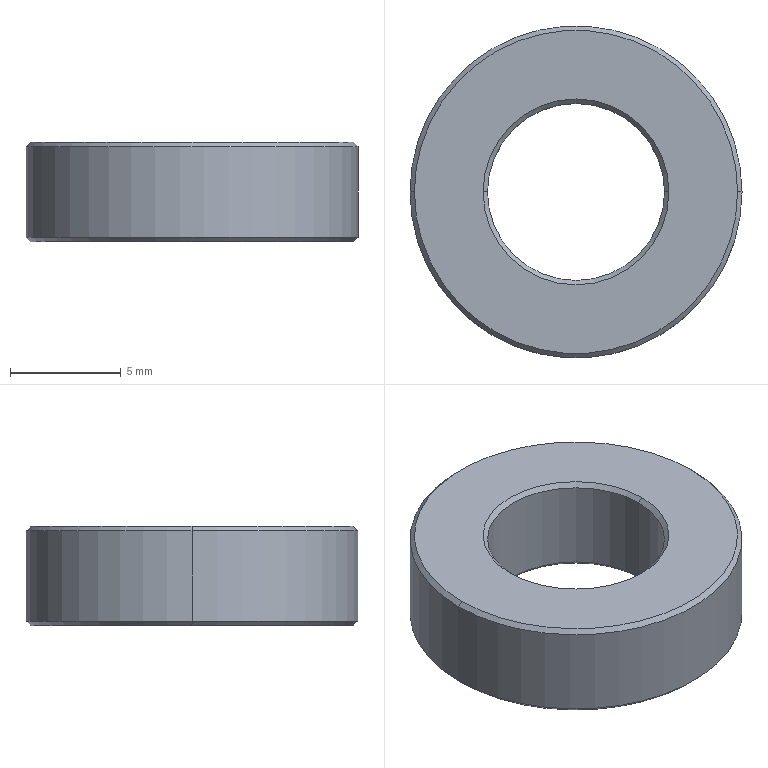Part | STEP file | 1 solid | 14 faces | box 15 x 15 x 4.5 mm | volume 566.131 mm3 | cone 8 | cylinder 4 | plane 2 | commonest cylinder face diameters 8 x2 15 x2
STEP:
#1=CARTESIAN_POINT('',(0.,0.,0.));
#2=DIRECTION('',(0.,0.,1.));
#3=DIRECTION('',(1.,0.,0.));
#4=AXIS2_PLACEMENT_3D('',#1,#2,#3);
#5=CARTESIAN_POINT('',(4.,0.,4.3));
#6=VERTEX_POINT('',#5);
#7=CARTESIAN_POINT('',(4.2,0.,4.5));
#8=VERTEX_POINT('',#7);
#9=CARTESIAN_POINT('',(4.,0.,4.3));
#10=DIRECTION('',(0.7071,0.,0.7071));
#11=VECTOR('',#10,1.);
#12=LINE('',#9,#11);
#13=CARTESIAN_POINT('',(0.,0.,4.3));
#14=DIRECTION('',(0.,0.,1.));
#15=DIRECTION('',(1.,0.,0.));
#16=AXIS2_PLACEMENT_3D('',#13,#14,#15);
#17=CONICAL_SURFACE('',#16,4.,0.7854);
#18=CARTESIAN_POINT('',(6.283,0.));
#19=DIRECTION('',(0.,1.));
#20=VECTOR('',#19,1.);
#21=LINE('',#18,#20);
#22=(GEOMETRIC_REPRESENTATION_CONTEXT(2)PARAMETRIC_REPRESENTATION_CONTEXT()REPRESENTATION_CONTEXT('',''));
#23=DEFINITIONAL_REPRESENTATION('',(#21),#22);
#24=PCURVE('',#17,#23);
#25=CARTESIAN_POINT('',(0.,0.,4.3));
#26=DIRECTION('',(0.,0.,1.));
#27=DIRECTION('',(1.,0.,0.));
#28=AXIS2_PLACEMENT_3D('',#25,#26,#27);
#29=CONICAL_SURFACE('',#28,4.,0.7854);
#30=CARTESIAN_POINT('',(0.,0.));
#31=DIRECTION('',(0.,1.));
#32=VECTOR('',#31,1.);
#33=LINE('',#30,#32);
#34=(GEOMETRIC_REPRESENTATION_CONTEXT(2)PARAMETRIC_REPRESENTATION_CONTEXT()REPRESENTATION_CONTEXT('',''));
#35=DEFINITIONAL_REPRESENTATION('',(#33),#34);
#36=PCURVE('',#29,#35);
#37=SURFACE_CURVE('',#12,(#24,#36),.PCURVE_S1.);
#38=EDGE_CURVE('',#6,#8,#37,.T.);
#39=ORIENTED_EDGE('',*,*,#38,.T.);
#40=CARTESIAN_POINT('',(-4.2,0.,4.5));
#41=VERTEX_POINT('',#40);
#42=CARTESIAN_POINT('',(0.,0.,4.5));
#43=DIRECTION('',(0.,0.,-1.));
#44=DIRECTION('',(1.,0.,0.));
#45=AXIS2_PLACEMENT_3D('',#42,#43,#44);
#46=CIRCLE('',#45,4.2);
#47=CARTESIAN_POINT('',(6.283,0.2));
#48=DIRECTION('',(-1.,0.));
#49=VECTOR('',#48,1.);
#50=LINE('',#47,#49);
#51=(GEOMETRIC_REPRESENTATION_CONTEXT(2)PARAMETRIC_REPRESENTATION_CONTEXT()REPRESENTATION_CONTEXT('',''));
#52=DEFINITIONAL_REPRESENTATION('',(#50),#51);
#53=PCURVE('',#17,#52);
#54=CARTESIAN_POINT('',(0.,0.,4.5));
#55=DIRECTION('',(0.,0.,1.));
#56=DIRECTION('',(1.,0.,0.));
#57=AXIS2_PLACEMENT_3D('',#54,#55,#56);
#58=PLANE('',#57);
#59=CARTESIAN_POINT('',(4.2,0.));
#60=CARTESIAN_POINT('',(4.2,-7.275));
#61=CARTESIAN_POINT('',(-2.1,-3.637));
#62=CARTESIAN_POINT('',(-8.4,0.));
#63=CARTESIAN_POINT('',(-2.1,3.637));
#64=CARTESIAN_POINT('',(4.2,7.275));
#65=CARTESIAN_POINT('',(4.2,0.));
#66=(BOUNDED_CURVE()B_SPLINE_CURVE(2,(#59,#60,#61,#62,#63,#64,#65),.UNSPECIFIED.,.T.,.F.)B_SPLINE_CURVE_WITH_KNOTS((1,2,2,2,2,1),(-2.094,0.,2.094,4.189,6.283,8.378),.UNSPECIFIED.)CURVE()GEOMETRIC_REPRESENTATION_ITEM()RATIONAL_B_SPLINE_CURVE((1.,0.5,1.,0.5,1.,0.5,1.))REPRESENTATION_ITEM(''));
#67=(GEOMETRIC_REPRESENTATION_CONTEXT(2)PARAMETRIC_REPRESENTATION_CONTEXT()REPRESENTATION_CONTEXT('',''));
#68=DEFINITIONAL_REPRESENTATION('',(#66),#67);
#69=PCURVE('',#58,#68);
#70=SURFACE_CURVE('',#46,(#53,#69),.PCURVE_S1.);
#71=EDGE_CURVE('',#8,#41,#70,.T.);
#72=ORIENTED_EDGE('',*,*,#71,.T.);
#73=CARTESIAN_POINT('',(-4.,0.,4.3));
#74=VERTEX_POINT('',#73);
#75=CARTESIAN_POINT('',(-4.,0.,4.3));
#76=DIRECTION('',(-0.7071,0.,0.7071));
#77=VECTOR('',#76,1.);
#78=LINE('',#75,#77);
#79=CARTESIAN_POINT('',(3.142,0.));
#80=DIRECTION('',(0.,1.));
#81=VECTOR('',#80,1.);
#82=LINE('',#79,#81);
#83=(GEOMETRIC_REPRESENTATION_CONTEXT(2)PARAMETRIC_REPRESENTATION_CONTEXT()REPRESENTATION_CONTEXT('',''));
#84=DEFINITIONAL_REPRESENTATION('',(#82),#83);
#85=PCURVE('',#17,#84);
#86=CARTESIAN_POINT('',(3.142,0.));
#87=DIRECTION('',(0.,1.));
#88=VECTOR('',#87,1.);
#89=LINE('',#86,#88);
#90=(GEOMETRIC_REPRESENTATION_CONTEXT(2)PARAMETRIC_REPRESENTATION_CONTEXT()REPRESENTATION_CONTEXT('',''));
#91=DEFINITIONAL_REPRESENTATION('',(#89),#90);
#92=PCURVE('',#29,#91);
#93=SURFACE_CURVE('',#78,(#85,#92),.PCURVE_S1.);
#94=EDGE_CURVE('',#74,#41,#93,.T.);
#95=ORIENTED_EDGE('',*,*,#94,.F.);
#96=CARTESIAN_POINT('',(0.,0.,4.3));
#97=DIRECTION('',(0.,0.,1.));
#98=DIRECTION('',(1.,0.,0.));
#99=AXIS2_PLACEMENT_3D('',#96,#97,#98);
#100=CIRCLE('',#99,4.);
#101=CARTESIAN_POINT('',(0.,0.));
#102=DIRECTION('',(1.,0.));
#103=VECTOR('',#102,1.);
#104=LINE('',#101,#103);
#105=(GEOMETRIC_REPRESENTATION_CONTEXT(2)PARAMETRIC_REPRESENTATION_CONTEXT()REPRESENTATION_CONTEXT('',''));
#106=DEFINITIONAL_REPRESENTATION('',(#104),#105);
#107=PCURVE('',#17,#106);
#108=CARTESIAN_POINT('',(0.,0.,4.5));
#109=DIRECTION('',(0.,0.,-1.));
#110=DIRECTION('',(-1.,0.,0.));
#111=AXIS2_PLACEMENT_3D('',#108,#109,#110);
#112=CYLINDRICAL_SURFACE('',#111,4.);
#113=CARTESIAN_POINT('',(9.425,0.2));
#114=DIRECTION('',(-1.,0.));
#115=VECTOR('',#114,1.);
#116=LINE('',#113,#115);
#117=(GEOMETRIC_REPRESENTATION_CONTEXT(2)PARAMETRIC_REPRESENTATION_CONTEXT()REPRESENTATION_CONTEXT('',''));
#118=DEFINITIONAL_REPRESENTATION('',(#116),#117);
#119=PCURVE('',#112,#118);
#120=SURFACE_CURVE('',#100,(#107,#119),.PCURVE_S1.);
#121=EDGE_CURVE('',#74,#6,#120,.T.);
#122=ORIENTED_EDGE('',*,*,#121,.T.);
#123=EDGE_LOOP('',(#39,#72,#95,#122));
#124=FACE_BOUND('',#123,.F.);
#125=ADVANCED_FACE('',(#124),#17,.F.);
#126=CARTESIAN_POINT('',(7.3,0.,4.5));
#127=VERTEX_POINT('',#126);
#128=CARTESIAN_POINT('',(-7.3,0.,4.5));
#129=VERTEX_POINT('',#128);
#130=CARTESIAN_POINT('',(0.,0.,4.5));
#131=DIRECTION('',(0.,0.,1.));
#132=DIRECTION('',(1.,0.,0.));
#133=AXIS2_PLACEMENT_3D('',#130,#131,#132);
#134=CIRCLE('',#133,7.3);
#135=CARTESIAN_POINT('',(0.,0.,4.5));
#136=DIRECTION('',(0.,0.,-1.));
#137=DIRECTION('',(-1.,0.,0.));
#138=AXIS2_PLACEMENT_3D('',#135,#136,#137);
#139=CONICAL_SURFACE('',#138,7.3,0.7854);
#140=CARTESIAN_POINT('',(3.142,0.));
#141=DIRECTION('',(-1.,0.));
#142=VECTOR('',#141,1.);
#143=LINE('',#140,#142);
#144=(GEOMETRIC_REPRESENTATION_CONTEXT(2)PARAMETRIC_REPRESENTATION_CONTEXT()REPRESENTATION_CONTEXT('',''));
#145=DEFINITIONAL_REPRESENTATION('',(#143),#144);
#146=PCURVE('',#139,#145);
#147=CARTESIAN_POINT('',(0.,0.));
#148=DIRECTION('',(1.,0.));
#149=AXIS2_PLACEMENT_2D('',#147,#148);
#150=CIRCLE('',#149,7.3);
#151=(GEOMETRIC_REPRESENTATION_CONTEXT(2)PARAMETRIC_REPRESENTATION_CONTEXT()REPRESENTATION_CONTEXT('',''));
#152=DEFINITIONAL_REPRESENTATION('',(#150),#151);
#153=PCURVE('',#58,#152);
#154=SURFACE_CURVE('',#134,(#146,#153),.PCURVE_S1.);
#155=EDGE_CURVE('',#127,#129,#154,.T.);
#156=ORIENTED_EDGE('',*,*,#155,.F.);
#157=CARTESIAN_POINT('',(7.5,0.,4.3));
#158=VERTEX_POINT('',#157);
#159=CARTESIAN_POINT('',(7.3,0.,4.5));
#160=DIRECTION('',(0.7071,0.,-0.7071));
#161=VECTOR('',#160,1.);
#162=LINE('',#159,#161);
#163=CARTESIAN_POINT('',(3.142,0.));
#164=DIRECTION('',(0.,1.));
#165=VECTOR('',#164,1.);
#166=LINE('',#163,#165);
#167=(GEOMETRIC_REPRESENTATION_CONTEXT(2)PARAMETRIC_REPRESENTATION_CONTEXT()REPRESENTATION_CONTEXT('',''));
#168=DEFINITIONAL_REPRESENTATION('',(#166),#167);
#169=PCURVE('',#139,#168);
#170=CARTESIAN_POINT('',(0.,0.,4.5));
#171=DIRECTION('',(0.,0.,-1.));
#172=DIRECTION('',(-1.,0.,0.));
#173=AXIS2_PLACEMENT_3D('',#170,#171,#172);
#174=CONICAL_SURFACE('',#173,7.3,0.7854);
#175=CARTESIAN_POINT('',(3.142,0.));
#176=DIRECTION('',(0.,1.));
#177=VECTOR('',#176,1.);
#178=LINE('',#175,#177);
#179=(GEOMETRIC_REPRESENTATION_CONTEXT(2)PARAMETRIC_REPRESENTATION_CONTEXT()REPRESENTATION_CONTEXT('',''));
#180=DEFINITIONAL_REPRESENTATION('',(#178),#179);
#181=PCURVE('',#174,#180);
#182=SURFACE_CURVE('',#162,(#169,#181),.PCURVE_S1.);
#183=EDGE_CURVE('',#127,#158,#182,.T.);
#184=ORIENTED_EDGE('',*,*,#183,.T.);
#185=CARTESIAN_POINT('',(-7.5,0.,4.3));
#186=VERTEX_POINT('',#185);
#187=CARTESIAN_POINT('',(0.,0.,4.3));
#188=DIRECTION('',(0.,0.,-1.));
#189=DIRECTION('',(1.,0.,0.));
#190=AXIS2_PLACEMENT_3D('',#187,#188,#189);
#191=CIRCLE('',#190,7.5);
#192=CARTESIAN_POINT('',(-3.142,0.2));
#193=DIRECTION('',(1.,0.));
#194=VECTOR('',#193,1.);
#195=LINE('',#192,#194);
#196=(GEOMETRIC_REPRESENTATION_CONTEXT(2)PARAMETRIC_REPRESENTATION_CONTEXT()REPRESENTATION_CONTEXT('',''));
#197=DEFINITIONAL_REPRESENTATION('',(#195),#196);
#198=PCURVE('',#139,#197);
#199=CARTESIAN_POINT('',(0.,0.,4.5));
#200=DIRECTION('',(0.,0.,-1.));
#201=DIRECTION('',(-1.,0.,0.));
#202=AXIS2_PLACEMENT_3D('',#199,#200,#201);
#203=CYLINDRICAL_SURFACE('',#202,7.5);
#204=CARTESIAN_POINT('',(-3.142,0.2));
#205=DIRECTION('',(1.,0.));
#206=VECTOR('',#205,1.);
#207=LINE('',#204,#206);
#208=(GEOMETRIC_REPRESENTATION_CONTEXT(2)PARAMETRIC_REPRESENTATION_CONTEXT()REPRESENTATION_CONTEXT('',''));
#209=DEFINITIONAL_REPRESENTATION('',(#207),#208);
#210=PCURVE('',#203,#209);
#211=SURFACE_CURVE('',#191,(#198,#210),.PCURVE_S1.);
#212=EDGE_CURVE('',#186,#158,#211,.T.);
#213=ORIENTED_EDGE('',*,*,#212,.F.);
#214=CARTESIAN_POINT('',(-7.3,0.,4.5));
#215=DIRECTION('',(-0.7071,0.,-0.7071));
#216=VECTOR('',#215,1.);
#217=LINE('',#214,#216);
#218=CARTESIAN_POINT('',(0.,0.));
#219=DIRECTION('',(0.,1.));
#220=VECTOR('',#219,1.);
#221=LINE('',#218,#220);
#222=(GEOMETRIC_REPRESENTATION_CONTEXT(2)PARAMETRIC_REPRESENTATION_CONTEXT()REPRESENTATION_CONTEXT('',''));
#223=DEFINITIONAL_REPRESENTATION('',(#221),#222);
#224=PCURVE('',#139,#223);
#225=CARTESIAN_POINT('',(6.283,0.));
#226=DIRECTION('',(0.,1.));
#227=VECTOR('',#226,1.);
#228=LINE('',#225,#227);
#229=(GEOMETRIC_REPRESENTATION_CONTEXT(2)PARAMETRIC_REPRESENTATION_CONTEXT()REPRESENTATION_CONTEXT('',''));
#230=DEFINITIONAL_REPRESENTATION('',(#228),#229);
#231=PCURVE('',#174,#230);
#232=SURFACE_CURVE('',#217,(#224,#231),.PCURVE_S1.);
#233=EDGE_CURVE('',#129,#186,#232,.T.);
#234=ORIENTED_EDGE('',*,*,#233,.F.);
#235=EDGE_LOOP('',(#156,#184,#213,#234));
#236=FACE_BOUND('',#235,.T.);
#237=ADVANCED_FACE('',(#236),#139,.T.);
#238=CARTESIAN_POINT('',(-7.3,0.,0.));
#239=VERTEX_POINT('',#238);
#240=CARTESIAN_POINT('',(7.3,0.,0.));
#241=VERTEX_POINT('',#240);
#242=CARTESIAN_POINT('',(0.,0.,0.));
#243=DIRECTION('',(0.,0.,-1.));
#244=DIRECTION('',(1.,0.,0.));
#245=AXIS2_PLACEMENT_3D('',#242,#243,#244);
#246=CIRCLE('',#245,7.3);
#247=CARTESIAN_POINT('',(0.,0.,0.2));
#248=DIRECTION('',(0.,0.,1.));
#249=DIRECTION('',(1.,0.,0.));
#250=AXIS2_PLACEMENT_3D('',#247,#248,#249);
#251=CONICAL_SURFACE('',#250,7.5,0.7854);
#252=CARTESIAN_POINT('',(6.283,-0.2));
#253=DIRECTION('',(-1.,0.));
#254=VECTOR('',#253,1.);
#255=LINE('',#252,#254);
#256=(GEOMETRIC_REPRESENTATION_CONTEXT(2)PARAMETRIC_REPRESENTATION_CONTEXT()REPRESENTATION_CONTEXT('',''));
#257=DEFINITIONAL_REPRESENTATION('',(#255),#256);
#258=PCURVE('',#251,#257);
#259=CARTESIAN_POINT('',(0.,0.,0.));
#260=DIRECTION('',(0.,0.,1.));
#261=DIRECTION('',(1.,0.,0.));
#262=AXIS2_PLACEMENT_3D('',#259,#260,#261);
#263=PLANE('',#262);
#264=CARTESIAN_POINT('',(7.3,0.));
#265=CARTESIAN_POINT('',(7.3,-12.644));
#266=CARTESIAN_POINT('',(-3.65,-6.322));
#267=CARTESIAN_POINT('',(-14.6,0.));
#268=CARTESIAN_POINT('',(-3.65,6.322));
#269=CARTESIAN_POINT('',(7.3,12.644));
#270=CARTESIAN_POINT('',(7.3,0.));
#271=(BOUNDED_CURVE()B_SPLINE_CURVE(2,(#264,#265,#266,#267,#268,#269,#270),.UNSPECIFIED.,.T.,.F.)B_SPLINE_CURVE_WITH_KNOTS((1,2,2,2,2,1),(-2.094,0.,2.094,4.189,6.283,8.378),.UNSPECIFIED.)CURVE()GEOMETRIC_REPRESENTATION_ITEM()RATIONAL_B_SPLINE_CURVE((1.,0.5,1.,0.5,1.,0.5,1.))REPRESENTATION_ITEM(''));
#272=(GEOMETRIC_REPRESENTATION_CONTEXT(2)PARAMETRIC_REPRESENTATION_CONTEXT()REPRESENTATION_CONTEXT('',''));
#273=DEFINITIONAL_REPRESENTATION('',(#271),#272);
#274=PCURVE('',#263,#273);
#275=SURFACE_CURVE('',#246,(#258,#274),.PCURVE_S1.);
#276=EDGE_CURVE('',#239,#241,#275,.T.);
#277=ORIENTED_EDGE('',*,*,#276,.F.);
#278=CARTESIAN_POINT('',(-7.5,0.,0.2));
#279=VERTEX_POINT('',#278);
#280=CARTESIAN_POINT('',(-7.5,0.,0.2));
#281=DIRECTION('',(-0.7071,0.,0.7071));
#282=VECTOR('',#281,1.);
#283=LINE('',#280,#282);
#284=CARTESIAN_POINT('',(3.142,0.));
#285=DIRECTION('',(0.,1.));
#286=VECTOR('',#285,1.);
#287=LINE('',#284,#286);
#288=(GEOMETRIC_REPRESENTATION_CONTEXT(2)PARAMETRIC_REPRESENTATION_CONTEXT()REPRESENTATION_CONTEXT('',''));
#289=DEFINITIONAL_REPRESENTATION('',(#287),#288);
#290=PCURVE('',#251,#289);
#291=CARTESIAN_POINT('',(0.,0.,0.2));
#292=DIRECTION('',(0.,0.,1.));
#293=DIRECTION('',(1.,0.,0.));
#294=AXIS2_PLACEMENT_3D('',#291,#292,#293);
#295=CONICAL_SURFACE('',#294,7.5,0.7854);
#296=CARTESIAN_POINT('',(3.142,0.));
#297=DIRECTION('',(0.,1.));
#298=VECTOR('',#297,1.);
#299=LINE('',#296,#298);
#300=(GEOMETRIC_REPRESENTATION_CONTEXT(2)PARAMETRIC_REPRESENTATION_CONTEXT()REPRESENTATION_CONTEXT('',''));
#301=DEFINITIONAL_REPRESENTATION('',(#299),#300);
#302=PCURVE('',#295,#301);
#303=SURFACE_CURVE('',#283,(#290,#302),.PCURVE_S1.);
#304=EDGE_CURVE('',#239,#279,#303,.T.);
#305=ORIENTED_EDGE('',*,*,#304,.T.);
#306=CARTESIAN_POINT('',(7.5,0.,0.2));
#307=VERTEX_POINT('',#306);
#308=CARTESIAN_POINT('',(0.,0.,0.2));
#309=DIRECTION('',(0.,0.,1.));
#310=DIRECTION('',(1.,0.,0.));
#311=AXIS2_PLACEMENT_3D('',#308,#309,#310);
#312=CIRCLE('',#311,7.5);
#313=CARTESIAN_POINT('',(0.,0.));
#314=DIRECTION('',(1.,0.));
#315=VECTOR('',#314,1.);
#316=LINE('',#313,#315);
#317=(GEOMETRIC_REPRESENTATION_CONTEXT(2)PARAMETRIC_REPRESENTATION_CONTEXT()REPRESENTATION_CONTEXT('',''));
#318=DEFINITIONAL_REPRESENTATION('',(#316),#317);
#319=PCURVE('',#251,#318);
#320=CARTESIAN_POINT('',(3.142,4.3));
#321=DIRECTION('',(-1.,0.));
#322=VECTOR('',#321,1.);
#323=LINE('',#320,#322);
#324=(GEOMETRIC_REPRESENTATION_CONTEXT(2)PARAMETRIC_REPRESENTATION_CONTEXT()REPRESENTATION_CONTEXT('',''));
#325=DEFINITIONAL_REPRESENTATION('',(#323),#324);
#326=PCURVE('',#203,#325);
#327=SURFACE_CURVE('',#312,(#319,#326),.PCURVE_S1.);
#328=EDGE_CURVE('',#307,#279,#327,.T.);
#329=ORIENTED_EDGE('',*,*,#328,.F.);
#330=CARTESIAN_POINT('',(7.5,0.,0.2));
#331=DIRECTION('',(0.7071,0.,0.7071));
#332=VECTOR('',#331,1.);
#333=LINE('',#330,#332);
#334=CARTESIAN_POINT('',(0.,0.));
#335=DIRECTION('',(0.,1.));
#336=VECTOR('',#335,1.);
#337=LINE('',#334,#336);
#338=(GEOMETRIC_REPRESENTATION_CONTEXT(2)PARAMETRIC_REPRESENTATION_CONTEXT()REPRESENTATION_CONTEXT('',''));
#339=DEFINITIONAL_REPRESENTATION('',(#337),#338);
#340=PCURVE('',#251,#339);
#341=CARTESIAN_POINT('',(6.283,0.));
#342=DIRECTION('',(0.,1.));
#343=VECTOR('',#342,1.);
#344=LINE('',#341,#343);
#345=(GEOMETRIC_REPRESENTATION_CONTEXT(2)PARAMETRIC_REPRESENTATION_CONTEXT()REPRESENTATION_CONTEXT('',''));
#346=DEFINITIONAL_REPRESENTATION('',(#344),#345);
#347=PCURVE('',#295,#346);
#348=SURFACE_CURVE('',#333,(#340,#347),.PCURVE_S1.);
#349=EDGE_CURVE('',#241,#307,#348,.T.);
#350=ORIENTED_EDGE('',*,*,#349,.F.);
#351=EDGE_LOOP('',(#277,#305,#329,#350));
#352=FACE_BOUND('',#351,.T.);
#353=ADVANCED_FACE('',(#352),#251,.T.);
#354=CARTESIAN_POINT('',(-4.,0.,0.2));
#355=VERTEX_POINT('',#354);
#356=CARTESIAN_POINT('',(-4.2,0.,0.));
#357=VERTEX_POINT('',#356);
#358=CARTESIAN_POINT('',(-4.2,0.,0.));
#359=DIRECTION('',(-0.7071,0.,-0.7071));
#360=VECTOR('',#359,1.);
#361=LINE('',#358,#360);
#362=CARTESIAN_POINT('',(0.,0.,0.));
#363=DIRECTION('',(0.,0.,-1.));
#364=DIRECTION('',(-1.,0.,0.));
#365=AXIS2_PLACEMENT_3D('',#362,#363,#364);
#366=CONICAL_SURFACE('',#365,4.2,0.7854);
#367=CARTESIAN_POINT('',(6.283,0.));
#368=DIRECTION('',(0.,1.));
#369=VECTOR('',#368,1.);
#370=LINE('',#367,#369);
#371=(GEOMETRIC_REPRESENTATION_CONTEXT(2)PARAMETRIC_REPRESENTATION_CONTEXT()REPRESENTATION_CONTEXT('',''));
#372=DEFINITIONAL_REPRESENTATION('',(#370),#371);
#373=PCURVE('',#366,#372);
#374=CARTESIAN_POINT('',(0.,0.,0.));
#375=DIRECTION('',(0.,0.,-1.));
#376=DIRECTION('',(-1.,0.,0.));
#377=AXIS2_PLACEMENT_3D('',#374,#375,#376);
#378=CONICAL_SURFACE('',#377,4.2,0.7854);
#379=CARTESIAN_POINT('',(0.,0.));
#380=DIRECTION('',(0.,1.));
#381=VECTOR('',#380,1.);
#382=LINE('',#379,#381);
#383=(GEOMETRIC_REPRESENTATION_CONTEXT(2)PARAMETRIC_REPRESENTATION_CONTEXT()REPRESENTATION_CONTEXT('',''));
#384=DEFINITIONAL_REPRESENTATION('',(#382),#383);
#385=PCURVE('',#378,#384);
#386=SURFACE_CURVE('',#361,(#373,#385),.PCURVE_S1.);
#387=EDGE_CURVE('',#355,#357,#386,.T.);
#388=ORIENTED_EDGE('',*,*,#387,.T.);
#389=CARTESIAN_POINT('',(4.2,0.,0.));
#390=VERTEX_POINT('',#389);
#391=CARTESIAN_POINT('',(0.,0.,0.));
#392=DIRECTION('',(0.,0.,1.));
#393=DIRECTION('',(1.,0.,0.));
#394=AXIS2_PLACEMENT_3D('',#391,#392,#393);
#395=CIRCLE('',#394,4.2);
#396=CARTESIAN_POINT('',(9.425,0.));
#397=DIRECTION('',(-1.,0.));
#398=VECTOR('',#397,1.);
#399=LINE('',#396,#398);
#400=(GEOMETRIC_REPRESENTATION_CONTEXT(2)PARAMETRIC_REPRESENTATION_CONTEXT()REPRESENTATION_CONTEXT('',''));
#401=DEFINITIONAL_REPRESENTATION('',(#399),#400);
#402=PCURVE('',#366,#401);
#403=CARTESIAN_POINT('',(0.,0.));
#404=DIRECTION('',(1.,0.));
#405=AXIS2_PLACEMENT_2D('',#403,#404);
#406=CIRCLE('',#405,4.2);
#407=(GEOMETRIC_REPRESENTATION_CONTEXT(2)PARAMETRIC_REPRESENTATION_CONTEXT()REPRESENTATION_CONTEXT('',''));
#408=DEFINITIONAL_REPRESENTATION('',(#406),#407);
#409=PCURVE('',#263,#408);
#410=SURFACE_CURVE('',#395,(#402,#409),.PCURVE_S1.);
#411=EDGE_CURVE('',#357,#390,#410,.T.);
#412=ORIENTED_EDGE('',*,*,#411,.T.);
#413=CARTESIAN_POINT('',(4.,0.,0.2));
#414=VERTEX_POINT('',#413);
#415=CARTESIAN_POINT('',(4.2,0.,0.));
#416=DIRECTION('',(0.7071,0.,-0.7071));
#417=VECTOR('',#416,1.);
#418=LINE('',#415,#417);
#419=CARTESIAN_POINT('',(3.142,0.));
#420=DIRECTION('',(0.,1.));
#421=VECTOR('',#420,1.);
#422=LINE('',#419,#421);
#423=(GEOMETRIC_REPRESENTATION_CONTEXT(2)PARAMETRIC_REPRESENTATION_CONTEXT()REPRESENTATION_CONTEXT('',''));
#424=DEFINITIONAL_REPRESENTATION('',(#422),#423);
#425=PCURVE('',#366,#424);
#426=CARTESIAN_POINT('',(3.142,0.));
#427=DIRECTION('',(0.,1.));
#428=VECTOR('',#427,1.);
#429=LINE('',#426,#428);
#430=(GEOMETRIC_REPRESENTATION_CONTEXT(2)PARAMETRIC_REPRESENTATION_CONTEXT()REPRESENTATION_CONTEXT('',''));
#431=DEFINITIONAL_REPRESENTATION('',(#429),#430);
#432=PCURVE('',#378,#431);
#433=SURFACE_CURVE('',#418,(#425,#432),.PCURVE_S1.);
#434=EDGE_CURVE('',#414,#390,#433,.T.);
#435=ORIENTED_EDGE('',*,*,#434,.F.);
#436=CARTESIAN_POINT('',(0.,0.,0.2));
#437=DIRECTION('',(0.,0.,-1.));
#438=DIRECTION('',(1.,0.,0.));
#439=AXIS2_PLACEMENT_3D('',#436,#437,#438);
#440=CIRCLE('',#439,4.);
#441=CARTESIAN_POINT('',(3.142,-0.2));
#442=DIRECTION('',(1.,0.));
#443=VECTOR('',#442,1.);
#444=LINE('',#441,#443);
#445=(GEOMETRIC_REPRESENTATION_CONTEXT(2)PARAMETRIC_REPRESENTATION_CONTEXT()REPRESENTATION_CONTEXT('',''));
#446=DEFINITIONAL_REPRESENTATION('',(#444),#445);
#447=PCURVE('',#366,#446);
#448=CARTESIAN_POINT('',(3.142,4.3));
#449=DIRECTION('',(1.,0.));
#450=VECTOR('',#449,1.);
#451=LINE('',#448,#450);
#452=(GEOMETRIC_REPRESENTATION_CONTEXT(2)PARAMETRIC_REPRESENTATION_CONTEXT()REPRESENTATION_CONTEXT('',''));
#453=DEFINITIONAL_REPRESENTATION('',(#451),#452);
#454=PCURVE('',#112,#453);
#455=SURFACE_CURVE('',#440,(#447,#454),.PCURVE_S1.);
#456=EDGE_CURVE('',#414,#355,#455,.T.);
#457=ORIENTED_EDGE('',*,*,#456,.T.);
#458=EDGE_LOOP('',(#388,#412,#435,#457));
#459=FACE_BOUND('',#458,.F.);
#460=ADVANCED_FACE('',(#459),#366,.F.);
#461=CARTESIAN_POINT('',(-4.,0.,4.5));
#462=DIRECTION('',(0.,0.,-1.));
#463=VECTOR('',#462,1.);
#464=LINE('',#461,#463);
#465=CARTESIAN_POINT('',(6.283,0.));
#466=DIRECTION('',(0.,1.));
#467=VECTOR('',#466,1.);
#468=LINE('',#465,#467);
#469=(GEOMETRIC_REPRESENTATION_CONTEXT(2)PARAMETRIC_REPRESENTATION_CONTEXT()REPRESENTATION_CONTEXT('',''));
#470=DEFINITIONAL_REPRESENTATION('',(#468),#469);
#471=PCURVE('',#112,#470);
#472=CARTESIAN_POINT('',(0.,0.,4.5));
#473=DIRECTION('',(0.,0.,-1.));
#474=DIRECTION('',(-1.,0.,0.));
#475=AXIS2_PLACEMENT_3D('',#472,#473,#474);
#476=CYLINDRICAL_SURFACE('',#475,4.);
#477=CARTESIAN_POINT('',(0.,0.));
#478=DIRECTION('',(0.,1.));
#479=VECTOR('',#478,1.);
#480=LINE('',#477,#479);
#481=(GEOMETRIC_REPRESENTATION_CONTEXT(2)PARAMETRIC_REPRESENTATION_CONTEXT()REPRESENTATION_CONTEXT('',''));
#482=DEFINITIONAL_REPRESENTATION('',(#480),#481);
#483=PCURVE('',#476,#482);
#484=SURFACE_CURVE('',#464,(#471,#483),.PCURVE_S1.);
#485=EDGE_CURVE('',#74,#355,#484,.T.);
#486=ORIENTED_EDGE('',*,*,#485,.T.);
#487=ORIENTED_EDGE('',*,*,#456,.F.);
#488=CARTESIAN_POINT('',(4.,0.,4.5));
#489=DIRECTION('',(0.,0.,-1.));
#490=VECTOR('',#489,1.);
#491=LINE('',#488,#490);
#492=CARTESIAN_POINT('',(3.142,0.));
#493=DIRECTION('',(0.,1.));
#494=VECTOR('',#493,1.);
#495=LINE('',#492,#494);
#496=(GEOMETRIC_REPRESENTATION_CONTEXT(2)PARAMETRIC_REPRESENTATION_CONTEXT()REPRESENTATION_CONTEXT('',''));
#497=DEFINITIONAL_REPRESENTATION('',(#495),#496);
#498=PCURVE('',#112,#497);
#499=CARTESIAN_POINT('',(3.142,0.));
#500=DIRECTION('',(0.,1.));
#501=VECTOR('',#500,1.);
#502=LINE('',#499,#501);
#503=(GEOMETRIC_REPRESENTATION_CONTEXT(2)PARAMETRIC_REPRESENTATION_CONTEXT()REPRESENTATION_CONTEXT('',''));
#504=DEFINITIONAL_REPRESENTATION('',(#502),#503);
#505=PCURVE('',#476,#504);
#506=SURFACE_CURVE('',#491,(#498,#505),.PCURVE_S1.);
#507=EDGE_CURVE('',#6,#414,#506,.T.);
#508=ORIENTED_EDGE('',*,*,#507,.F.);
#509=ORIENTED_EDGE('',*,*,#121,.F.);
#510=EDGE_LOOP('',(#486,#487,#508,#509));
#511=FACE_BOUND('',#510,.F.);
#512=ADVANCED_FACE('',(#511),#112,.F.);
#513=ORIENTED_EDGE('',*,*,#212,.T.);
#514=CARTESIAN_POINT('',(7.5,0.,4.5));
#515=DIRECTION('',(0.,0.,-1.));
#516=VECTOR('',#515,1.);
#517=LINE('',#514,#516);
#518=CARTESIAN_POINT('',(3.142,0.));
#519=DIRECTION('',(0.,1.));
#520=VECTOR('',#519,1.);
#521=LINE('',#518,#520);
#522=(GEOMETRIC_REPRESENTATION_CONTEXT(2)PARAMETRIC_REPRESENTATION_CONTEXT()REPRESENTATION_CONTEXT('',''));
#523=DEFINITIONAL_REPRESENTATION('',(#521),#522);
#524=PCURVE('',#203,#523);
#525=CARTESIAN_POINT('',(0.,0.,4.5));
#526=DIRECTION('',(0.,0.,-1.));
#527=DIRECTION('',(-1.,0.,0.));
#528=AXIS2_PLACEMENT_3D('',#525,#526,#527);
#529=CYLINDRICAL_SURFACE('',#528,7.5);
#530=CARTESIAN_POINT('',(3.142,0.));
#531=DIRECTION('',(0.,1.));
#532=VECTOR('',#531,1.);
#533=LINE('',#530,#532);
#534=(GEOMETRIC_REPRESENTATION_CONTEXT(2)PARAMETRIC_REPRESENTATION_CONTEXT()REPRESENTATION_CONTEXT('',''));
#535=DEFINITIONAL_REPRESENTATION('',(#533),#534);
#536=PCURVE('',#529,#535);
#537=SURFACE_CURVE('',#517,(#524,#536),.PCURVE_S1.);
#538=EDGE_CURVE('',#158,#307,#537,.T.);
#539=ORIENTED_EDGE('',*,*,#538,.T.);
#540=ORIENTED_EDGE('',*,*,#328,.T.);
#541=CARTESIAN_POINT('',(-7.5,0.,4.5));
#542=DIRECTION('',(0.,0.,-1.));
#543=VECTOR('',#542,1.);
#544=LINE('',#541,#543);
#545=CARTESIAN_POINT('',(0.,0.));
#546=DIRECTION('',(0.,1.));
#547=VECTOR('',#546,1.);
#548=LINE('',#545,#547);
#549=(GEOMETRIC_REPRESENTATION_CONTEXT(2)PARAMETRIC_REPRESENTATION_CONTEXT()REPRESENTATION_CONTEXT('',''));
#550=DEFINITIONAL_REPRESENTATION('',(#548),#549);
#551=PCURVE('',#203,#550);
#552=CARTESIAN_POINT('',(6.283,0.));
#553=DIRECTION('',(0.,1.));
#554=VECTOR('',#553,1.);
#555=LINE('',#552,#554);
#556=(GEOMETRIC_REPRESENTATION_CONTEXT(2)PARAMETRIC_REPRESENTATION_CONTEXT()REPRESENTATION_CONTEXT('',''));
#557=DEFINITIONAL_REPRESENTATION('',(#555),#556);
#558=PCURVE('',#529,#557);
#559=SURFACE_CURVE('',#544,(#551,#558),.PCURVE_S1.);
#560=EDGE_CURVE('',#186,#279,#559,.T.);
#561=ORIENTED_EDGE('',*,*,#560,.F.);
#562=EDGE_LOOP('',(#513,#539,#540,#561));
#563=FACE_BOUND('',#562,.T.);
#564=ADVANCED_FACE('',(#563),#203,.T.);
#565=CARTESIAN_POINT('',(0.,0.,4.5));
#566=DIRECTION('',(0.,0.,1.));
#567=DIRECTION('',(1.,0.,0.));
#568=AXIS2_PLACEMENT_3D('',#565,#566,#567);
#569=CIRCLE('',#568,7.3);
#570=CARTESIAN_POINT('',(0.,0.));
#571=DIRECTION('',(1.,0.));
#572=AXIS2_PLACEMENT_2D('',#570,#571);
#573=CIRCLE('',#572,7.3);
#574=(GEOMETRIC_REPRESENTATION_CONTEXT(2)PARAMETRIC_REPRESENTATION_CONTEXT()REPRESENTATION_CONTEXT('',''));
#575=DEFINITIONAL_REPRESENTATION('',(#573),#574);
#576=PCURVE('',#58,#575);
#577=CARTESIAN_POINT('',(9.425,0.));
#578=DIRECTION('',(-1.,0.));
#579=VECTOR('',#578,1.);
#580=LINE('',#577,#579);
#581=(GEOMETRIC_REPRESENTATION_CONTEXT(2)PARAMETRIC_REPRESENTATION_CONTEXT()REPRESENTATION_CONTEXT('',''));
#582=DEFINITIONAL_REPRESENTATION('',(#580),#581);
#583=PCURVE('',#174,#582);
#584=SURFACE_CURVE('',#569,(#576,#583),.PCURVE_S1.);
#585=EDGE_CURVE('',#129,#127,#584,.T.);
#586=ORIENTED_EDGE('',*,*,#585,.T.);
#587=ORIENTED_EDGE('',*,*,#155,.T.);
#588=EDGE_LOOP('',(#586,#587));
#589=FACE_BOUND('',#588,.T.);
#590=ORIENTED_EDGE('',*,*,#71,.T.);
#591=CARTESIAN_POINT('',(0.,0.,4.5));
#592=DIRECTION('',(0.,0.,-1.));
#593=DIRECTION('',(1.,0.,0.));
#594=AXIS2_PLACEMENT_3D('',#591,#592,#593);
#595=CIRCLE('',#594,4.2);
#596=CARTESIAN_POINT('',(4.2,0.));
#597=CARTESIAN_POINT('',(4.2,-7.275));
#598=CARTESIAN_POINT('',(-2.1,-3.637));
#599=CARTESIAN_POINT('',(-8.4,0.));
#600=CARTESIAN_POINT('',(-2.1,3.637));
#601=CARTESIAN_POINT('',(4.2,7.275));
#602=CARTESIAN_POINT('',(4.2,0.));
#603=(BOUNDED_CURVE()B_SPLINE_CURVE(2,(#596,#597,#598,#599,#600,#601,#602),.UNSPECIFIED.,.T.,.F.)B_SPLINE_CURVE_WITH_KNOTS((1,2,2,2,2,1),(-2.094,0.,2.094,4.189,6.283,8.378),.UNSPECIFIED.)CURVE()GEOMETRIC_REPRESENTATION_ITEM()RATIONAL_B_SPLINE_CURVE((1.,0.5,1.,0.5,1.,0.5,1.))REPRESENTATION_ITEM(''));
#604=(GEOMETRIC_REPRESENTATION_CONTEXT(2)PARAMETRIC_REPRESENTATION_CONTEXT()REPRESENTATION_CONTEXT('',''));
#605=DEFINITIONAL_REPRESENTATION('',(#603),#604);
#606=PCURVE('',#58,#605);
#607=CARTESIAN_POINT('',(6.283,0.2));
#608=DIRECTION('',(-1.,0.));
#609=VECTOR('',#608,1.);
#610=LINE('',#607,#609);
#611=(GEOMETRIC_REPRESENTATION_CONTEXT(2)PARAMETRIC_REPRESENTATION_CONTEXT()REPRESENTATION_CONTEXT('',''));
#612=DEFINITIONAL_REPRESENTATION('',(#610),#611);
#613=PCURVE('',#29,#612);
#614=SURFACE_CURVE('',#595,(#606,#613),.PCURVE_S1.);
#615=EDGE_CURVE('',#41,#8,#614,.T.);
#616=ORIENTED_EDGE('',*,*,#615,.T.);
#617=EDGE_LOOP('',(#590,#616));
#618=FACE_BOUND('',#617,.T.);
#619=ADVANCED_FACE('',(#589,#618),#58,.T.);
#620=ORIENTED_EDGE('',*,*,#411,.T.);
#621=CARTESIAN_POINT('',(0.,0.,0.));
#622=DIRECTION('',(0.,0.,1.));
#623=DIRECTION('',(1.,0.,0.));
#624=AXIS2_PLACEMENT_3D('',#621,#622,#623);
#625=CIRCLE('',#624,4.2);
#626=CARTESIAN_POINT('',(0.,0.));
#627=DIRECTION('',(1.,0.));
#628=AXIS2_PLACEMENT_2D('',#626,#627);
#629=CIRCLE('',#628,4.2);
#630=(GEOMETRIC_REPRESENTATION_CONTEXT(2)PARAMETRIC_REPRESENTATION_CONTEXT()REPRESENTATION_CONTEXT('',''));
#631=DEFINITIONAL_REPRESENTATION('',(#629),#630);
#632=PCURVE('',#263,#631);
#633=CARTESIAN_POINT('',(3.142,0.));
#634=DIRECTION('',(-1.,0.));
#635=VECTOR('',#634,1.);
#636=LINE('',#633,#635);
#637=(GEOMETRIC_REPRESENTATION_CONTEXT(2)PARAMETRIC_REPRESENTATION_CONTEXT()REPRESENTATION_CONTEXT('',''));
#638=DEFINITIONAL_REPRESENTATION('',(#636),#637);
#639=PCURVE('',#378,#638);
#640=SURFACE_CURVE('',#625,(#632,#639),.PCURVE_S1.);
#641=EDGE_CURVE('',#390,#357,#640,.T.);
#642=ORIENTED_EDGE('',*,*,#641,.T.);
#643=EDGE_LOOP('',(#620,#642));
#644=FACE_BOUND('',#643,.T.);
#645=CARTESIAN_POINT('',(0.,0.,0.));
#646=DIRECTION('',(0.,0.,-1.));
#647=DIRECTION('',(1.,0.,0.));
#648=AXIS2_PLACEMENT_3D('',#645,#646,#647);
#649=CIRCLE('',#648,7.3);
#650=CARTESIAN_POINT('',(7.3,0.));
#651=CARTESIAN_POINT('',(7.3,-12.644));
#652=CARTESIAN_POINT('',(-3.65,-6.322));
#653=CARTESIAN_POINT('',(-14.6,0.));
#654=CARTESIAN_POINT('',(-3.65,6.322));
#655=CARTESIAN_POINT('',(7.3,12.644));
#656=CARTESIAN_POINT('',(7.3,0.));
#657=(BOUNDED_CURVE()B_SPLINE_CURVE(2,(#650,#651,#652,#653,#654,#655,#656),.UNSPECIFIED.,.T.,.F.)B_SPLINE_CURVE_WITH_KNOTS((1,2,2,2,2,1),(-2.094,0.,2.094,4.189,6.283,8.378),.UNSPECIFIED.)CURVE()GEOMETRIC_REPRESENTATION_ITEM()RATIONAL_B_SPLINE_CURVE((1.,0.5,1.,0.5,1.,0.5,1.))REPRESENTATION_ITEM(''));
#658=(GEOMETRIC_REPRESENTATION_CONTEXT(2)PARAMETRIC_REPRESENTATION_CONTEXT()REPRESENTATION_CONTEXT('',''));
#659=DEFINITIONAL_REPRESENTATION('',(#657),#658);
#660=PCURVE('',#263,#659);
#661=CARTESIAN_POINT('',(6.283,-0.2));
#662=DIRECTION('',(-1.,0.));
#663=VECTOR('',#662,1.);
#664=LINE('',#661,#663);
#665=(GEOMETRIC_REPRESENTATION_CONTEXT(2)PARAMETRIC_REPRESENTATION_CONTEXT()REPRESENTATION_CONTEXT('',''));
#666=DEFINITIONAL_REPRESENTATION('',(#664),#665);
#667=PCURVE('',#295,#666);
#668=SURFACE_CURVE('',#649,(#660,#667),.PCURVE_S1.);
#669=EDGE_CURVE('',#241,#239,#668,.T.);
#670=ORIENTED_EDGE('',*,*,#669,.T.);
#671=ORIENTED_EDGE('',*,*,#276,.T.);
#672=EDGE_LOOP('',(#670,#671));
#673=FACE_BOUND('',#672,.T.);
#674=ADVANCED_FACE('',(#644,#673),#263,.F.);
#675=ORIENTED_EDGE('',*,*,#538,.F.);
#676=CARTESIAN_POINT('',(0.,0.,4.3));
#677=DIRECTION('',(0.,0.,-1.));
#678=DIRECTION('',(1.,0.,0.));
#679=AXIS2_PLACEMENT_3D('',#676,#677,#678);
#680=CIRCLE('',#679,7.5);
#681=CARTESIAN_POINT('',(3.142,0.2));
#682=DIRECTION('',(1.,0.));
#683=VECTOR('',#682,1.);
#684=LINE('',#681,#683);
#685=(GEOMETRIC_REPRESENTATION_CONTEXT(2)PARAMETRIC_REPRESENTATION_CONTEXT()REPRESENTATION_CONTEXT('',''));
#686=DEFINITIONAL_REPRESENTATION('',(#684),#685);
#687=PCURVE('',#529,#686);
#688=CARTESIAN_POINT('',(3.142,0.2));
#689=DIRECTION('',(1.,0.));
#690=VECTOR('',#689,1.);
#691=LINE('',#688,#690);
#692=(GEOMETRIC_REPRESENTATION_CONTEXT(2)PARAMETRIC_REPRESENTATION_CONTEXT()REPRESENTATION_CONTEXT('',''));
#693=DEFINITIONAL_REPRESENTATION('',(#691),#692);
#694=PCURVE('',#174,#693);
#695=SURFACE_CURVE('',#680,(#687,#694),.PCURVE_S1.);
#696=EDGE_CURVE('',#158,#186,#695,.T.);
#697=ORIENTED_EDGE('',*,*,#696,.T.);
#698=ORIENTED_EDGE('',*,*,#560,.T.);
#699=CARTESIAN_POINT('',(0.,0.,0.2));
#700=DIRECTION('',(0.,0.,1.));
#701=DIRECTION('',(1.,0.,0.));
#702=AXIS2_PLACEMENT_3D('',#699,#700,#701);
#703=CIRCLE('',#702,7.5);
#704=CARTESIAN_POINT('',(9.425,4.3));
#705=DIRECTION('',(-1.,0.));
#706=VECTOR('',#705,1.);
#707=LINE('',#704,#706);
#708=(GEOMETRIC_REPRESENTATION_CONTEXT(2)PARAMETRIC_REPRESENTATION_CONTEXT()REPRESENTATION_CONTEXT('',''));
#709=DEFINITIONAL_REPRESENTATION('',(#707),#708);
#710=PCURVE('',#529,#709);
#711=CARTESIAN_POINT('',(0.,0.));
#712=DIRECTION('',(1.,0.));
#713=VECTOR('',#712,1.);
#714=LINE('',#711,#713);
#715=(GEOMETRIC_REPRESENTATION_CONTEXT(2)PARAMETRIC_REPRESENTATION_CONTEXT()REPRESENTATION_CONTEXT('',''));
#716=DEFINITIONAL_REPRESENTATION('',(#714),#715);
#717=PCURVE('',#295,#716);
#718=SURFACE_CURVE('',#703,(#710,#717),.PCURVE_S1.);
#719=EDGE_CURVE('',#279,#307,#718,.T.);
#720=ORIENTED_EDGE('',*,*,#719,.T.);
#721=EDGE_LOOP('',(#675,#697,#698,#720));
#722=FACE_BOUND('',#721,.T.);
#723=ADVANCED_FACE('',(#722),#529,.T.);
#724=CARTESIAN_POINT('',(0.,0.,0.2));
#725=DIRECTION('',(0.,0.,-1.));
#726=DIRECTION('',(1.,0.,0.));
#727=AXIS2_PLACEMENT_3D('',#724,#725,#726);
#728=CIRCLE('',#727,4.);
#729=CARTESIAN_POINT('',(-3.142,4.3));
#730=DIRECTION('',(1.,0.));
#731=VECTOR('',#730,1.);
#732=LINE('',#729,#731);
#733=(GEOMETRIC_REPRESENTATION_CONTEXT(2)PARAMETRIC_REPRESENTATION_CONTEXT()REPRESENTATION_CONTEXT('',''));
#734=DEFINITIONAL_REPRESENTATION('',(#732),#733);
#735=PCURVE('',#476,#734);
#736=CARTESIAN_POINT('',(-3.142,-0.2));
#737=DIRECTION('',(1.,0.));
#738=VECTOR('',#737,1.);
#739=LINE('',#736,#738);
#740=(GEOMETRIC_REPRESENTATION_CONTEXT(2)PARAMETRIC_REPRESENTATION_CONTEXT()REPRESENTATION_CONTEXT('',''));
#741=DEFINITIONAL_REPRESENTATION('',(#739),#740);
#742=PCURVE('',#378,#741);
#743=SURFACE_CURVE('',#728,(#735,#742),.PCURVE_S1.);
#744=EDGE_CURVE('',#355,#414,#743,.T.);
#745=ORIENTED_EDGE('',*,*,#744,.F.);
#746=ORIENTED_EDGE('',*,*,#485,.F.);
#747=CARTESIAN_POINT('',(0.,0.,4.3));
#748=DIRECTION('',(0.,0.,1.));
#749=DIRECTION('',(1.,0.,0.));
#750=AXIS2_PLACEMENT_3D('',#747,#748,#749);
#751=CIRCLE('',#750,4.);
#752=CARTESIAN_POINT('',(3.142,0.2));
#753=DIRECTION('',(-1.,0.));
#754=VECTOR('',#753,1.);
#755=LINE('',#752,#754);
#756=(GEOMETRIC_REPRESENTATION_CONTEXT(2)PARAMETRIC_REPRESENTATION_CONTEXT()REPRESENTATION_CONTEXT('',''));
#757=DEFINITIONAL_REPRESENTATION('',(#755),#756);
#758=PCURVE('',#476,#757);
#759=CARTESIAN_POINT('',(0.,0.));
#760=DIRECTION('',(1.,0.));
#761=VECTOR('',#760,1.);
#762=LINE('',#759,#761);
#763=(GEOMETRIC_REPRESENTATION_CONTEXT(2)PARAMETRIC_REPRESENTATION_CONTEXT()REPRESENTATION_CONTEXT('',''));
#764=DEFINITIONAL_REPRESENTATION('',(#762),#763);
#765=PCURVE('',#29,#764);
#766=SURFACE_CURVE('',#751,(#758,#765),.PCURVE_S1.);
#767=EDGE_CURVE('',#6,#74,#766,.T.);
#768=ORIENTED_EDGE('',*,*,#767,.F.);
#769=ORIENTED_EDGE('',*,*,#507,.T.);
#770=EDGE_LOOP('',(#745,#746,#768,#769));
#771=FACE_BOUND('',#770,.F.);
#772=ADVANCED_FACE('',(#771),#476,.F.);
#773=ORIENTED_EDGE('',*,*,#641,.T.);
#774=ORIENTED_EDGE('',*,*,#387,.F.);
#775=ORIENTED_EDGE('',*,*,#744,.T.);
#776=ORIENTED_EDGE('',*,*,#434,.T.);
#777=EDGE_LOOP('',(#773,#774,#775,#776));
#778=FACE_BOUND('',#777,.F.);
#779=ADVANCED_FACE('',(#778),#378,.F.);
#780=ORIENTED_EDGE('',*,*,#304,.F.);
#781=ORIENTED_EDGE('',*,*,#669,.F.);
#782=ORIENTED_EDGE('',*,*,#349,.T.);
#783=ORIENTED_EDGE('',*,*,#719,.F.);
#784=EDGE_LOOP('',(#780,#781,#782,#783));
#785=FACE_BOUND('',#784,.T.);
#786=ADVANCED_FACE('',(#785),#295,.T.);
#787=ORIENTED_EDGE('',*,*,#183,.F.);
#788=ORIENTED_EDGE('',*,*,#585,.F.);
#789=ORIENTED_EDGE('',*,*,#233,.T.);
#790=ORIENTED_EDGE('',*,*,#696,.F.);
#791=EDGE_LOOP('',(#787,#788,#789,#790));
#792=FACE_BOUND('',#791,.T.);
#793=ADVANCED_FACE('',(#792),#174,.T.);
#794=ORIENTED_EDGE('',*,*,#615,.T.);
#795=ORIENTED_EDGE('',*,*,#38,.F.);
#796=ORIENTED_EDGE('',*,*,#767,.T.);
#797=ORIENTED_EDGE('',*,*,#94,.T.);
#798=EDGE_LOOP('',(#794,#795,#796,#797));
#799=FACE_BOUND('',#798,.F.);
#800=ADVANCED_FACE('',(#799),#29,.F.);
#801=CLOSED_SHELL('',(#125,#237,#353,#460,#512,#564,#619,#674,#723,#772,#779,#786,#793,#800));
#802=MANIFOLD_SOLID_BREP('',#801);
#803=(LENGTH_UNIT()NAMED_UNIT(*)SI_UNIT(.MILLI.,.METRE.));
#804=UNCERTAINTY_MEASURE_WITH_UNIT(LENGTH_MEASURE(0.0000001),#803,'','');
#805=(NAMED_UNIT(*)PLANE_ANGLE_UNIT()SI_UNIT($,.RADIAN.));
#806=(NAMED_UNIT(*)SI_UNIT($,.STERADIAN.)SOLID_ANGLE_UNIT());
#807=(GEOMETRIC_REPRESENTATION_CONTEXT(3)GLOBAL_UNCERTAINTY_ASSIGNED_CONTEXT((#804))GLOBAL_UNIT_ASSIGNED_CONTEXT((#803,#805,#806))REPRESENTATION_CONTEXT('',''));
#808=ADVANCED_BREP_SHAPE_REPRESENTATION('',(#4,#802),#807);